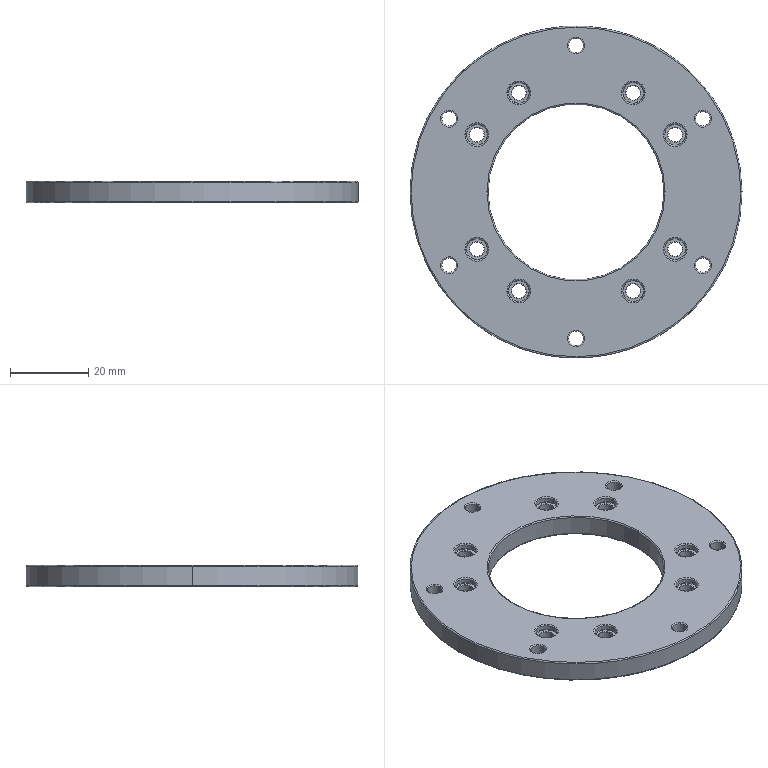Part | SolidWorks | features ICE 3, Fillet 2, Extrusion 1 | 1 solid | 184 faces | box 85 x 85 x 5.5 mm | volume 21445 mm3 | torus 120 | cylinder 48 | plane 16 | commonest cylinder face diameters 3.7 x28 5.5 x16 45 x2 85 x2